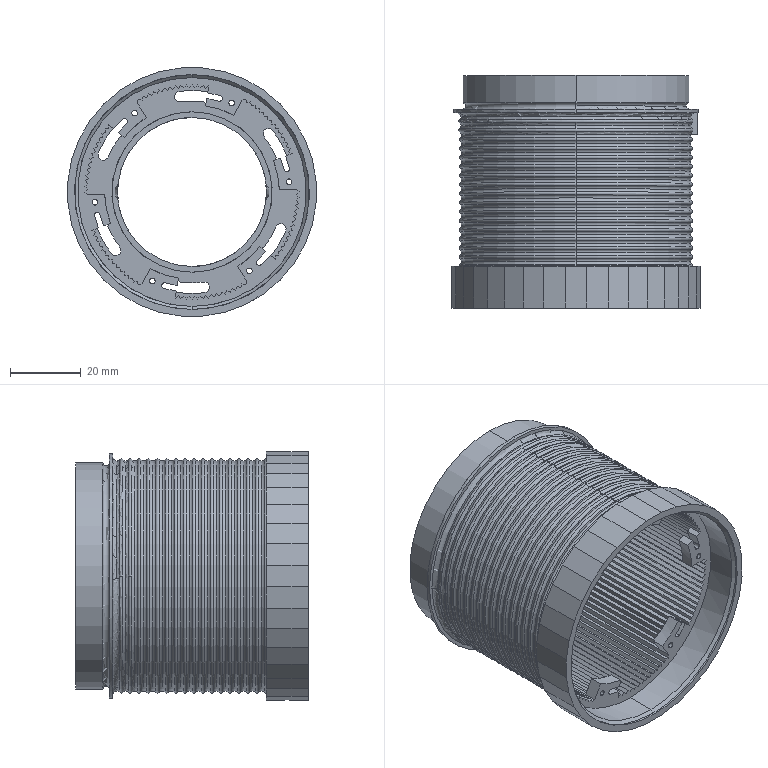Part | STEP file | 1 solid | 542 faces | box 70 x 65.6 x 70 mm | volume 40502 mm3 | plane 346 | torus 107 | cylinder 84 | cone 4 | spline 1 | commonest cylinder face diameters 1.6 x21 49.2 x12 3 x9 51.2 x7 57.2 x7 53.4 x6